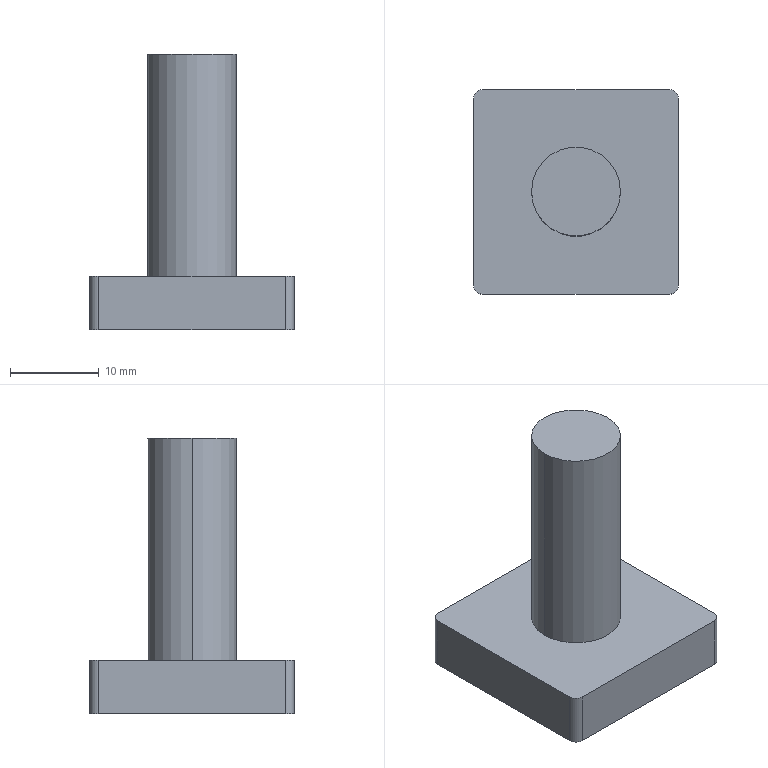Part | SolidWorks | features Extrusion 1, Fillet 1, ICE 1 | 1 solid | 13 faces | box 23 x 23 x 31 mm | volume 5132 mm3 | plane 7 | cylinder 6 | commonest cylinder face diameters 2 x4 10 x2
STEP:
#1=CARTESIAN_POINT('',(5.,0.,25.));
#2=VERTEX_POINT('',#1);
#3=CARTESIAN_POINT('',(-5.,0.,25.));
#4=VERTEX_POINT('',#3);
#5=CARTESIAN_POINT('',(0.,0.,25.));
#6=DIRECTION('',(0.,0.,1.));
#7=DIRECTION('',(1.,0.,0.));
#8=AXIS2_PLACEMENT_3D('',#5,#6,#7);
#9=CIRCLE('',#8,5.);
#10=EDGE_CURVE('',#2,#4,#9,.T.);
#11=ORIENTED_EDGE('',*,*,#10,.F.);
#12=CARTESIAN_POINT('',(5.,0.,0.));
#13=VERTEX_POINT('',#12);
#14=CARTESIAN_POINT('',(5.,0.,25.));
#15=DIRECTION('',(0.,0.,-1.));
#16=VECTOR('',#15,1000.);
#17=LINE('',#14,#16);
#18=EDGE_CURVE('',#2,#13,#17,.T.);
#19=ORIENTED_EDGE('',*,*,#18,.T.);
#20=CARTESIAN_POINT('',(-5.,0.,0.));
#21=VERTEX_POINT('',#20);
#22=CARTESIAN_POINT('',(0.,0.,0.));
#23=DIRECTION('',(0.,0.,1.));
#24=DIRECTION('',(1.,0.,0.));
#25=AXIS2_PLACEMENT_3D('',#22,#23,#24);
#26=CIRCLE('',#25,5.);
#27=EDGE_CURVE('',#13,#21,#26,.T.);
#28=ORIENTED_EDGE('',*,*,#27,.T.);
#29=CARTESIAN_POINT('',(-5.,0.,25.));
#30=DIRECTION('',(0.,0.,-1.));
#31=VECTOR('',#30,1000.);
#32=LINE('',#29,#31);
#33=EDGE_CURVE('',#4,#21,#32,.T.);
#34=ORIENTED_EDGE('',*,*,#33,.F.);
#35=EDGE_LOOP('',(#11,#19,#28,#34));
#36=FACE_OUTER_BOUND('',#35,.T.);
#37=CARTESIAN_POINT('',(0.,0.,25.));
#38=DIRECTION('',(0.,0.,-1.));
#39=DIRECTION('',(-1.,0.,0.));
#40=AXIS2_PLACEMENT_3D('',#37,#38,#39);
#41=CYLINDRICAL_SURFACE('',#40,5.);
#42=ADVANCED_FACE('',(#36),#41,.T.);
#43=ORIENTED_EDGE('',*,*,#18,.F.);
#44=CARTESIAN_POINT('',(0.,0.,25.));
#45=DIRECTION('',(0.,0.,1.));
#46=DIRECTION('',(1.,0.,0.));
#47=AXIS2_PLACEMENT_3D('',#44,#45,#46);
#48=CIRCLE('',#47,5.);
#49=EDGE_CURVE('',#4,#2,#48,.T.);
#50=ORIENTED_EDGE('',*,*,#49,.F.);
#51=ORIENTED_EDGE('',*,*,#33,.T.);
#52=CARTESIAN_POINT('',(0.,0.,0.));
#53=DIRECTION('',(0.,0.,1.));
#54=DIRECTION('',(1.,0.,0.));
#55=AXIS2_PLACEMENT_3D('',#52,#53,#54);
#56=CIRCLE('',#55,5.);
#57=EDGE_CURVE('',#21,#13,#56,.T.);
#58=ORIENTED_EDGE('',*,*,#57,.T.);
#59=EDGE_LOOP('',(#43,#50,#51,#58));
#60=FACE_OUTER_BOUND('',#59,.T.);
#61=CARTESIAN_POINT('',(0.,0.,25.));
#62=DIRECTION('',(0.,0.,-1.));
#63=DIRECTION('',(-1.,0.,0.));
#64=AXIS2_PLACEMENT_3D('',#61,#62,#63);
#65=CYLINDRICAL_SURFACE('',#64,5.);
#66=ADVANCED_FACE('',(#60),#65,.T.);
#67=ORIENTED_EDGE('',*,*,#49,.T.);
#68=ORIENTED_EDGE('',*,*,#10,.T.);
#69=EDGE_LOOP('',(#67,#68));
#70=FACE_OUTER_BOUND('',#69,.T.);
#71=CARTESIAN_POINT('',(0.,0.,25.));
#72=DIRECTION('',(0.,0.,1.));
#73=DIRECTION('',(1.,0.,0.));
#74=AXIS2_PLACEMENT_3D('',#71,#72,#73);
#75=PLANE('',#74);
#76=ADVANCED_FACE('',(#70),#75,.T.);
#77=CARTESIAN_POINT('',(-10.5,11.5,0.));
#78=VERTEX_POINT('',#77);
#79=CARTESIAN_POINT('',(10.5,11.5,0.));
#80=VERTEX_POINT('',#79);
#81=CARTESIAN_POINT('',(-11.5,11.5,0.));
#82=DIRECTION('',(1.,0.,0.));
#83=VECTOR('',#82,1000.);
#84=LINE('',#81,#83);
#85=EDGE_CURVE('',#78,#80,#84,.T.);
#86=ORIENTED_EDGE('',*,*,#85,.F.);
#87=CARTESIAN_POINT('',(-11.5,10.5,0.));
#88=VERTEX_POINT('',#87);
#89=CARTESIAN_POINT('',(-10.5,10.5,0.));
#90=DIRECTION('',(0.,0.,1.));
#91=DIRECTION('',(1.,0.,0.));
#92=AXIS2_PLACEMENT_3D('',#89,#90,#91);
#93=CIRCLE('',#92,1.);
#94=EDGE_CURVE('',#78,#88,#93,.T.);
#95=ORIENTED_EDGE('',*,*,#94,.T.);
#96=CARTESIAN_POINT('',(-11.5,-10.5,0.));
#97=VERTEX_POINT('',#96);
#98=CARTESIAN_POINT('',(-11.5,11.5,0.));
#99=DIRECTION('',(0.,1.,0.));
#100=VECTOR('',#99,1000.);
#101=LINE('',#98,#100);
#102=EDGE_CURVE('',#97,#88,#101,.T.);
#103=ORIENTED_EDGE('',*,*,#102,.F.);
#104=CARTESIAN_POINT('',(-10.5,-11.5,0.));
#105=VERTEX_POINT('',#104);
#106=CARTESIAN_POINT('',(-10.5,-10.5,0.));
#107=DIRECTION('',(0.,0.,1.));
#108=DIRECTION('',(1.,0.,0.));
#109=AXIS2_PLACEMENT_3D('',#106,#107,#108);
#110=CIRCLE('',#109,1.);
#111=EDGE_CURVE('',#97,#105,#110,.T.);
#112=ORIENTED_EDGE('',*,*,#111,.T.);
#113=CARTESIAN_POINT('',(10.5,-11.5,0.));
#114=VERTEX_POINT('',#113);
#115=CARTESIAN_POINT('',(-11.5,-11.5,0.));
#116=DIRECTION('',(-1.,0.,0.));
#117=VECTOR('',#116,1000.);
#118=LINE('',#115,#117);
#119=EDGE_CURVE('',#114,#105,#118,.T.);
#120=ORIENTED_EDGE('',*,*,#119,.F.);
#121=CARTESIAN_POINT('',(11.5,-10.5,0.));
#122=VERTEX_POINT('',#121);
#123=CARTESIAN_POINT('',(10.5,-10.5,0.));
#124=DIRECTION('',(0.,0.,1.));
#125=DIRECTION('',(1.,0.,0.));
#126=AXIS2_PLACEMENT_3D('',#123,#124,#125);
#127=CIRCLE('',#126,1.);
#128=EDGE_CURVE('',#114,#122,#127,.T.);
#129=ORIENTED_EDGE('',*,*,#128,.T.);
#130=CARTESIAN_POINT('',(11.5,10.5,0.));
#131=VERTEX_POINT('',#130);
#132=CARTESIAN_POINT('',(11.5,11.5,0.));
#133=DIRECTION('',(0.,-1.,0.));
#134=VECTOR('',#133,1000.);
#135=LINE('',#132,#134);
#136=EDGE_CURVE('',#131,#122,#135,.T.);
#137=ORIENTED_EDGE('',*,*,#136,.F.);
#138=CARTESIAN_POINT('',(10.5,10.5,0.));
#139=DIRECTION('',(0.,0.,1.));
#140=DIRECTION('',(1.,0.,0.));
#141=AXIS2_PLACEMENT_3D('',#138,#139,#140);
#142=CIRCLE('',#141,1.);
#143=EDGE_CURVE('',#131,#80,#142,.T.);
#144=ORIENTED_EDGE('',*,*,#143,.T.);
#145=EDGE_LOOP('',(#86,#95,#103,#112,#120,#129,#137,#144));
#146=FACE_OUTER_BOUND('',#145,.T.);
#147=ORIENTED_EDGE('',*,*,#57,.F.);
#148=ORIENTED_EDGE('',*,*,#27,.F.);
#149=EDGE_LOOP('',(#147,#148));
#150=FACE_BOUND('',#149,.T.);
#151=CARTESIAN_POINT('',(0.,0.,0.));
#152=DIRECTION('',(0.,0.,1.));
#153=DIRECTION('',(1.,0.,0.));
#154=AXIS2_PLACEMENT_3D('',#151,#152,#153);
#155=PLANE('',#154);
#156=ADVANCED_FACE('',(#146,#150),#155,.T.);
#157=CARTESIAN_POINT('',(11.5,10.5,-6.));
#158=VERTEX_POINT('',#157);
#159=CARTESIAN_POINT('',(11.5,-10.5,-6.));
#160=VERTEX_POINT('',#159);
#161=CARTESIAN_POINT('',(11.5,11.5,-6.));
#162=DIRECTION('',(0.,-1.,0.));
#163=VECTOR('',#162,1000.);
#164=LINE('',#161,#163);
#165=EDGE_CURVE('',#158,#160,#164,.T.);
#166=ORIENTED_EDGE('',*,*,#165,.F.);
#167=CARTESIAN_POINT('',(11.5,10.5,-6.));
#168=DIRECTION('',(0.,0.,1.));
#169=VECTOR('',#168,1000.);
#170=LINE('',#167,#169);
#171=EDGE_CURVE('',#158,#131,#170,.T.);
#172=ORIENTED_EDGE('',*,*,#171,.T.);
#173=ORIENTED_EDGE('',*,*,#136,.T.);
#174=CARTESIAN_POINT('',(11.5,-10.5,-6.));
#175=DIRECTION('',(0.,0.,-1.));
#176=VECTOR('',#175,1000.);
#177=LINE('',#174,#176);
#178=EDGE_CURVE('',#122,#160,#177,.T.);
#179=ORIENTED_EDGE('',*,*,#178,.T.);
#180=EDGE_LOOP('',(#166,#172,#173,#179));
#181=FACE_OUTER_BOUND('',#180,.T.);
#182=CARTESIAN_POINT('',(11.5,11.5,-6.));
#183=DIRECTION('',(-1.,0.,0.));
#184=DIRECTION('',(0.,-1.,0.));
#185=AXIS2_PLACEMENT_3D('',#182,#183,#184);
#186=PLANE('',#185);
#187=ADVANCED_FACE('',(#181),#186,.F.);
#188=ORIENTED_EDGE('',*,*,#119,.T.);
#189=CARTESIAN_POINT('',(-10.5,-11.5,-6.));
#190=VERTEX_POINT('',#189);
#191=CARTESIAN_POINT('',(-10.5,-11.5,-6.));
#192=DIRECTION('',(0.,0.,-1.));
#193=VECTOR('',#192,1000.);
#194=LINE('',#191,#193);
#195=EDGE_CURVE('',#105,#190,#194,.T.);
#196=ORIENTED_EDGE('',*,*,#195,.T.);
#197=CARTESIAN_POINT('',(10.5,-11.5,-6.));
#198=VERTEX_POINT('',#197);
#199=CARTESIAN_POINT('',(-11.5,-11.5,-6.));
#200=DIRECTION('',(-1.,0.,0.));
#201=VECTOR('',#200,1000.);
#202=LINE('',#199,#201);
#203=EDGE_CURVE('',#198,#190,#202,.T.);
#204=ORIENTED_EDGE('',*,*,#203,.F.);
#205=CARTESIAN_POINT('',(10.5,-11.5,-6.));
#206=DIRECTION('',(0.,0.,1.));
#207=VECTOR('',#206,1000.);
#208=LINE('',#205,#207);
#209=EDGE_CURVE('',#198,#114,#208,.T.);
#210=ORIENTED_EDGE('',*,*,#209,.T.);
#211=EDGE_LOOP('',(#188,#196,#204,#210));
#212=FACE_OUTER_BOUND('',#211,.T.);
#213=CARTESIAN_POINT('',(-11.5,-11.5,-6.));
#214=DIRECTION('',(0.,1.,0.));
#215=DIRECTION('',(-1.,0.,0.));
#216=AXIS2_PLACEMENT_3D('',#213,#214,#215);
#217=PLANE('',#216);
#218=ADVANCED_FACE('',(#212),#217,.F.);
#219=ORIENTED_EDGE('',*,*,#102,.T.);
#220=CARTESIAN_POINT('',(-11.5,10.5,-6.));
#221=VERTEX_POINT('',#220);
#222=CARTESIAN_POINT('',(-11.5,10.5,-6.));
#223=DIRECTION('',(0.,0.,-1.));
#224=VECTOR('',#223,1000.);
#225=LINE('',#222,#224);
#226=EDGE_CURVE('',#88,#221,#225,.T.);
#227=ORIENTED_EDGE('',*,*,#226,.T.);
#228=CARTESIAN_POINT('',(-11.5,-10.5,-6.));
#229=VERTEX_POINT('',#228);
#230=CARTESIAN_POINT('',(-11.5,11.5,-6.));
#231=DIRECTION('',(0.,1.,0.));
#232=VECTOR('',#231,1000.);
#233=LINE('',#230,#232);
#234=EDGE_CURVE('',#229,#221,#233,.T.);
#235=ORIENTED_EDGE('',*,*,#234,.F.);
#236=CARTESIAN_POINT('',(-11.5,-10.5,-6.));
#237=DIRECTION('',(0.,0.,1.));
#238=VECTOR('',#237,1000.);
#239=LINE('',#236,#238);
#240=EDGE_CURVE('',#229,#97,#239,.T.);
#241=ORIENTED_EDGE('',*,*,#240,.T.);
#242=EDGE_LOOP('',(#219,#227,#235,#241));
#243=FACE_OUTER_BOUND('',#242,.T.);
#244=CARTESIAN_POINT('',(-11.5,11.5,-6.));
#245=DIRECTION('',(1.,0.,0.));
#246=DIRECTION('',(0.,1.,0.));
#247=AXIS2_PLACEMENT_3D('',#244,#245,#246);
#248=PLANE('',#247);
#249=ADVANCED_FACE('',(#243),#248,.F.);
#250=CARTESIAN_POINT('',(-10.5,11.5,-6.));
#251=VERTEX_POINT('',#250);
#252=CARTESIAN_POINT('',(10.5,11.5,-6.));
#253=VERTEX_POINT('',#252);
#254=CARTESIAN_POINT('',(-11.5,11.5,-6.));
#255=DIRECTION('',(1.,0.,0.));
#256=VECTOR('',#255,1000.);
#257=LINE('',#254,#256);
#258=EDGE_CURVE('',#251,#253,#257,.T.);
#259=ORIENTED_EDGE('',*,*,#258,.F.);
#260=CARTESIAN_POINT('',(-10.5,11.5,-6.));
#261=DIRECTION('',(0.,0.,1.));
#262=VECTOR('',#261,1000.);
#263=LINE('',#260,#262);
#264=EDGE_CURVE('',#251,#78,#263,.T.);
#265=ORIENTED_EDGE('',*,*,#264,.T.);
#266=ORIENTED_EDGE('',*,*,#85,.T.);
#267=CARTESIAN_POINT('',(10.5,11.5,-6.));
#268=DIRECTION('',(0.,0.,-1.));
#269=VECTOR('',#268,1000.);
#270=LINE('',#267,#269);
#271=EDGE_CURVE('',#80,#253,#270,.T.);
#272=ORIENTED_EDGE('',*,*,#271,.T.);
#273=EDGE_LOOP('',(#259,#265,#266,#272));
#274=FACE_OUTER_BOUND('',#273,.T.);
#275=CARTESIAN_POINT('',(-11.5,11.5,-6.));
#276=DIRECTION('',(0.,-1.,0.));
#277=DIRECTION('',(1.,0.,0.));
#278=AXIS2_PLACEMENT_3D('',#275,#276,#277);
#279=PLANE('',#278);
#280=ADVANCED_FACE('',(#274),#279,.F.);
#281=ORIENTED_EDGE('',*,*,#234,.T.);
#282=CARTESIAN_POINT('',(-10.5,10.5,-6.));
#283=DIRECTION('',(0.,0.,-1.));
#284=DIRECTION('',(1.,0.,0.));
#285=AXIS2_PLACEMENT_3D('',#282,#283,#284);
#286=CIRCLE('',#285,1.);
#287=EDGE_CURVE('',#221,#251,#286,.T.);
#288=ORIENTED_EDGE('',*,*,#287,.T.);
#289=ORIENTED_EDGE('',*,*,#258,.T.);
#290=CARTESIAN_POINT('',(10.5,10.5,-6.));
#291=DIRECTION('',(0.,0.,-1.));
#292=DIRECTION('',(1.,0.,0.));
#293=AXIS2_PLACEMENT_3D('',#290,#291,#292);
#294=CIRCLE('',#293,1.);
#295=EDGE_CURVE('',#253,#158,#294,.T.);
#296=ORIENTED_EDGE('',*,*,#295,.T.);
#297=ORIENTED_EDGE('',*,*,#165,.T.);
#298=CARTESIAN_POINT('',(10.5,-10.5,-6.));
#299=DIRECTION('',(0.,0.,-1.));
#300=DIRECTION('',(1.,0.,0.));
#301=AXIS2_PLACEMENT_3D('',#298,#299,#300);
#302=CIRCLE('',#301,1.);
#303=EDGE_CURVE('',#160,#198,#302,.T.);
#304=ORIENTED_EDGE('',*,*,#303,.T.);
#305=ORIENTED_EDGE('',*,*,#203,.T.);
#306=CARTESIAN_POINT('',(-10.5,-10.5,-6.));
#307=DIRECTION('',(0.,0.,-1.));
#308=DIRECTION('',(1.,0.,0.));
#309=AXIS2_PLACEMENT_3D('',#306,#307,#308);
#310=CIRCLE('',#309,1.);
#311=EDGE_CURVE('',#190,#229,#310,.T.);
#312=ORIENTED_EDGE('',*,*,#311,.T.);
#313=EDGE_LOOP('',(#281,#288,#289,#296,#297,#304,#305,#312));
#314=FACE_OUTER_BOUND('',#313,.T.);
#315=CARTESIAN_POINT('',(0.,0.,-6.));
#316=DIRECTION('',(0.,0.,1.));
#317=DIRECTION('',(1.,0.,0.));
#318=AXIS2_PLACEMENT_3D('',#315,#316,#317);
#319=PLANE('',#318);
#320=ADVANCED_FACE('',(#314),#319,.F.);
#321=ORIENTED_EDGE('',*,*,#287,.F.);
#322=ORIENTED_EDGE('',*,*,#226,.F.);
#323=ORIENTED_EDGE('',*,*,#94,.F.);
#324=ORIENTED_EDGE('',*,*,#264,.F.);
#325=EDGE_LOOP('',(#321,#322,#323,#324));
#326=FACE_OUTER_BOUND('',#325,.T.);
#327=CARTESIAN_POINT('',(-10.5,10.5,-6.));
#328=DIRECTION('',(0.,0.,1.));
#329=DIRECTION('',(1.,0.,0.));
#330=AXIS2_PLACEMENT_3D('',#327,#328,#329);
#331=CYLINDRICAL_SURFACE('',#330,1.);
#332=ADVANCED_FACE('',(#326),#331,.T.);
#333=ORIENTED_EDGE('',*,*,#311,.F.);
#334=ORIENTED_EDGE('',*,*,#195,.F.);
#335=ORIENTED_EDGE('',*,*,#111,.F.);
#336=ORIENTED_EDGE('',*,*,#240,.F.);
#337=EDGE_LOOP('',(#333,#334,#335,#336));
#338=FACE_OUTER_BOUND('',#337,.T.);
#339=CARTESIAN_POINT('',(-10.5,-10.5,-6.));
#340=DIRECTION('',(0.,0.,1.));
#341=DIRECTION('',(1.,0.,0.));
#342=AXIS2_PLACEMENT_3D('',#339,#340,#341);
#343=CYLINDRICAL_SURFACE('',#342,1.);
#344=ADVANCED_FACE('',(#338),#343,.T.);
#345=ORIENTED_EDGE('',*,*,#295,.F.);
#346=ORIENTED_EDGE('',*,*,#271,.F.);
#347=ORIENTED_EDGE('',*,*,#143,.F.);
#348=ORIENTED_EDGE('',*,*,#171,.F.);
#349=EDGE_LOOP('',(#345,#346,#347,#348));
#350=FACE_OUTER_BOUND('',#349,.T.);
#351=CARTESIAN_POINT('',(10.5,10.5,-6.));
#352=DIRECTION('',(0.,0.,1.));
#353=DIRECTION('',(1.,0.,0.));
#354=AXIS2_PLACEMENT_3D('',#351,#352,#353);
#355=CYLINDRICAL_SURFACE('',#354,1.);
#356=ADVANCED_FACE('',(#350),#355,.T.);
#357=ORIENTED_EDGE('',*,*,#303,.F.);
#358=ORIENTED_EDGE('',*,*,#178,.F.);
#359=ORIENTED_EDGE('',*,*,#128,.F.);
#360=ORIENTED_EDGE('',*,*,#209,.F.);
#361=EDGE_LOOP('',(#357,#358,#359,#360));
#362=FACE_OUTER_BOUND('',#361,.T.);
#363=CARTESIAN_POINT('',(10.5,-10.5,-6.));
#364=DIRECTION('',(0.,0.,1.));
#365=DIRECTION('',(1.,0.,0.));
#366=AXIS2_PLACEMENT_3D('',#363,#364,#365);
#367=CYLINDRICAL_SURFACE('',#366,1.);
#368=ADVANCED_FACE('',(#362),#367,.T.);
#369=CLOSED_SHELL('',(#42,#66,#76,#156,#187,#218,#249,#280,#320,#332,#344,#356,#368));
#370=MANIFOLD_SOLID_BREP('',#369);
#371=CARTESIAN_POINT('',(0.,0.,0.));
#372=DIRECTION('',(0.,0.,1.));
#373=DIRECTION('',(1.,0.,0.));
#374=AXIS2_PLACEMENT_3D('',#371,#372,#373);
#375=(LENGTH_UNIT()NAMED_UNIT(*)SI_UNIT(.MILLI.,.METRE.));
#376=UNCERTAINTY_MEASURE_WITH_UNIT(LENGTH_MEASURE(0.00001),#375,'','');
#377=(NAMED_UNIT(*)PLANE_ANGLE_UNIT()SI_UNIT($,.RADIAN.));
#378=(NAMED_UNIT(*)SI_UNIT($,.STERADIAN.)SOLID_ANGLE_UNIT());
#379=(GEOMETRIC_REPRESENTATION_CONTEXT(3)GLOBAL_UNCERTAINTY_ASSIGNED_CONTEXT((#376))GLOBAL_UNIT_ASSIGNED_CONTEXT((#375,#377,#378))REPRESENTATION_CONTEXT('',''));
#380=ADVANCED_BREP_SHAPE_REPRESENTATION('',(#370,#374),#379);